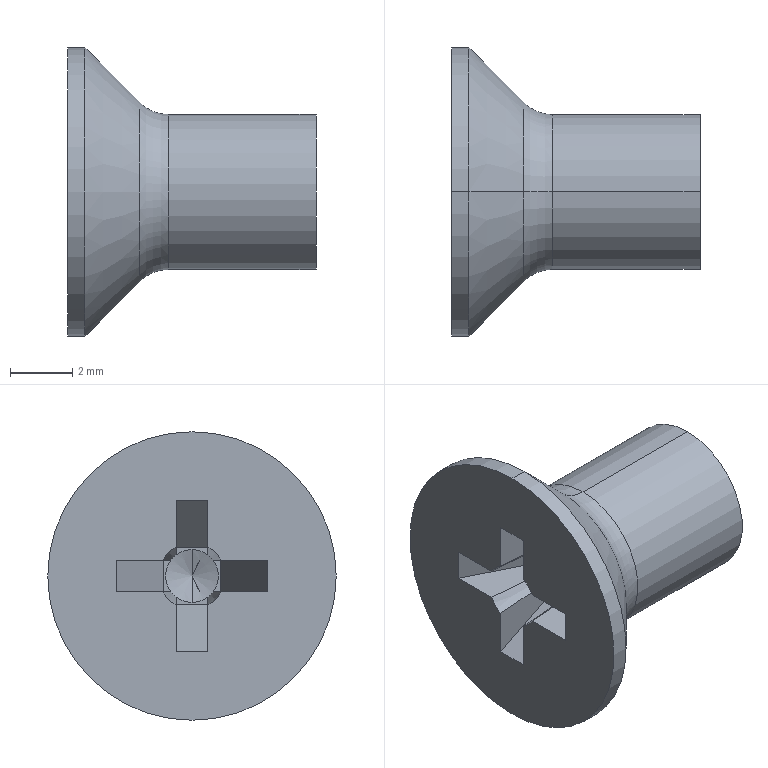Part | STEP file | countersunk flat head cross recess screw_din_ISO 7046-1 - M5 x 8 - Z --- 8N | 1 solid | 32 faces | box 8 x 9.3 x 9.3 mm | volume 212.099 mm3 | plane 18 | cone 8 | cylinder 4 | torus 2 | commonest cylinder face diameters 5 x2 9.3 x2